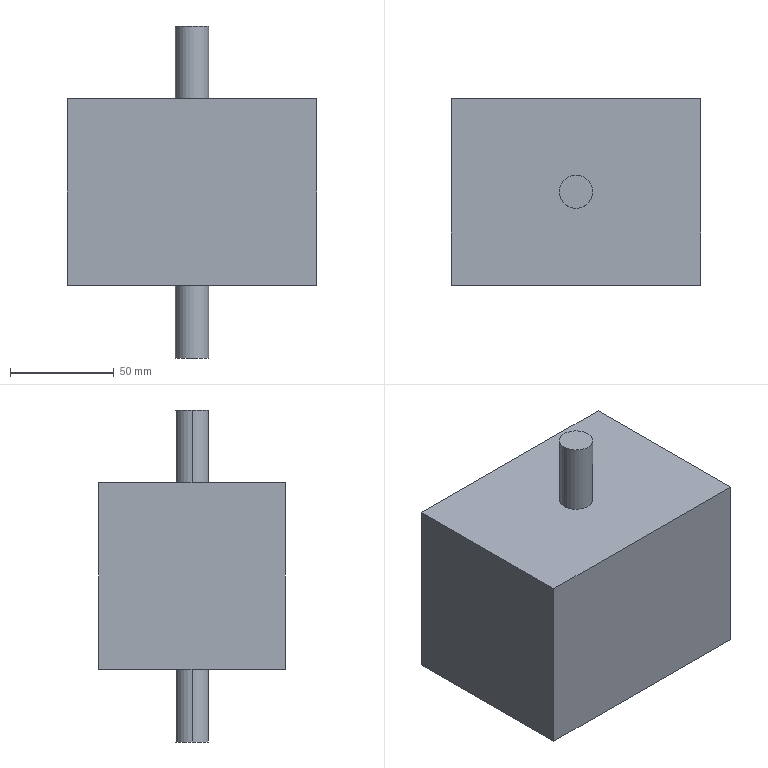Part | SolidWorks | features Extrusion 1, ICE 1 | 1 solid | 12 faces | box 120 x 90 x 160 mm | volume 986074 mm3 | plane 8 | cylinder 4 | commonest cylinder face diameters 16 x4
STEP:
#1=CARTESIAN_POINT('',(8.,0.,-80.));
#2=VERTEX_POINT('',#1);
#3=CARTESIAN_POINT('',(-8.,0.,-80.));
#4=VERTEX_POINT('',#3);
#5=CARTESIAN_POINT('',(0.,0.,-80.));
#6=DIRECTION('',(0.,0.,1.));
#7=DIRECTION('',(1.,0.,0.));
#8=AXIS2_PLACEMENT_3D('',#5,#6,#7);
#9=CIRCLE('',#8,8.);
#10=EDGE_CURVE('',#2,#4,#9,.T.);
#11=ORIENTED_EDGE('',*,*,#10,.T.);
#12=CARTESIAN_POINT('',(-8.,0.,-45.));
#13=VERTEX_POINT('',#12);
#14=CARTESIAN_POINT('',(-8.,0.,-80.));
#15=DIRECTION('',(0.,0.,1.));
#16=VECTOR('',#15,1000.);
#17=LINE('',#14,#16);
#18=EDGE_CURVE('',#4,#13,#17,.T.);
#19=ORIENTED_EDGE('',*,*,#18,.T.);
#20=CARTESIAN_POINT('',(8.,0.,-45.));
#21=VERTEX_POINT('',#20);
#22=CARTESIAN_POINT('',(0.,0.,-45.));
#23=DIRECTION('',(0.,0.,1.));
#24=DIRECTION('',(1.,0.,0.));
#25=AXIS2_PLACEMENT_3D('',#22,#23,#24);
#26=CIRCLE('',#25,8.);
#27=EDGE_CURVE('',#21,#13,#26,.T.);
#28=ORIENTED_EDGE('',*,*,#27,.F.);
#29=CARTESIAN_POINT('',(8.,0.,-80.));
#30=DIRECTION('',(0.,0.,1.));
#31=VECTOR('',#30,1000.);
#32=LINE('',#29,#31);
#33=EDGE_CURVE('',#2,#21,#32,.T.);
#34=ORIENTED_EDGE('',*,*,#33,.F.);
#35=EDGE_LOOP('',(#11,#19,#28,#34));
#36=FACE_OUTER_BOUND('',#35,.T.);
#37=CARTESIAN_POINT('',(0.,0.,-80.));
#38=DIRECTION('',(0.,0.,1.));
#39=DIRECTION('',(1.,0.,0.));
#40=AXIS2_PLACEMENT_3D('',#37,#38,#39);
#41=CYLINDRICAL_SURFACE('',#40,8.);
#42=ADVANCED_FACE('',(#36),#41,.T.);
#43=CARTESIAN_POINT('',(8.,0.,45.));
#44=VERTEX_POINT('',#43);
#45=CARTESIAN_POINT('',(-8.,0.,45.));
#46=VERTEX_POINT('',#45);
#47=CARTESIAN_POINT('',(0.,0.,45.));
#48=DIRECTION('',(0.,0.,1.));
#49=DIRECTION('',(1.,0.,0.));
#50=AXIS2_PLACEMENT_3D('',#47,#48,#49);
#51=CIRCLE('',#50,8.);
#52=EDGE_CURVE('',#44,#46,#51,.T.);
#53=ORIENTED_EDGE('',*,*,#52,.T.);
#54=CARTESIAN_POINT('',(-8.,0.,80.));
#55=VERTEX_POINT('',#54);
#56=CARTESIAN_POINT('',(-8.,0.,-80.));
#57=DIRECTION('',(0.,0.,1.));
#58=VECTOR('',#57,1000.);
#59=LINE('',#56,#58);
#60=EDGE_CURVE('',#46,#55,#59,.T.);
#61=ORIENTED_EDGE('',*,*,#60,.T.);
#62=CARTESIAN_POINT('',(8.,0.,80.));
#63=VERTEX_POINT('',#62);
#64=CARTESIAN_POINT('',(0.,0.,80.));
#65=DIRECTION('',(0.,0.,1.));
#66=DIRECTION('',(1.,0.,0.));
#67=AXIS2_PLACEMENT_3D('',#64,#65,#66);
#68=CIRCLE('',#67,8.);
#69=EDGE_CURVE('',#63,#55,#68,.T.);
#70=ORIENTED_EDGE('',*,*,#69,.F.);
#71=CARTESIAN_POINT('',(8.,0.,-80.));
#72=DIRECTION('',(0.,0.,1.));
#73=VECTOR('',#72,1000.);
#74=LINE('',#71,#73);
#75=EDGE_CURVE('',#44,#63,#74,.T.);
#76=ORIENTED_EDGE('',*,*,#75,.F.);
#77=EDGE_LOOP('',(#53,#61,#70,#76));
#78=FACE_OUTER_BOUND('',#77,.T.);
#79=CARTESIAN_POINT('',(0.,0.,-80.));
#80=DIRECTION('',(0.,0.,1.));
#81=DIRECTION('',(1.,0.,0.));
#82=AXIS2_PLACEMENT_3D('',#79,#80,#81);
#83=CYLINDRICAL_SURFACE('',#82,8.);
#84=ADVANCED_FACE('',(#78),#83,.T.);
#85=CARTESIAN_POINT('',(-60.,45.,45.));
#86=VERTEX_POINT('',#85);
#87=CARTESIAN_POINT('',(-60.,-45.,45.));
#88=VERTEX_POINT('',#87);
#89=CARTESIAN_POINT('',(-60.,45.,45.));
#90=DIRECTION('',(0.,-1.,0.));
#91=VECTOR('',#90,1000.);
#92=LINE('',#89,#91);
#93=EDGE_CURVE('',#86,#88,#92,.T.);
#94=ORIENTED_EDGE('',*,*,#93,.F.);
#95=CARTESIAN_POINT('',(-60.,45.,-45.));
#96=VERTEX_POINT('',#95);
#97=CARTESIAN_POINT('',(-60.,45.,-45.));
#98=DIRECTION('',(0.,0.,1.));
#99=VECTOR('',#98,1000.);
#100=LINE('',#97,#99);
#101=EDGE_CURVE('',#96,#86,#100,.T.);
#102=ORIENTED_EDGE('',*,*,#101,.F.);
#103=CARTESIAN_POINT('',(-60.,-45.,-45.));
#104=VERTEX_POINT('',#103);
#105=CARTESIAN_POINT('',(-60.,45.,-45.));
#106=DIRECTION('',(0.,-1.,0.));
#107=VECTOR('',#106,1000.);
#108=LINE('',#105,#107);
#109=EDGE_CURVE('',#96,#104,#108,.T.);
#110=ORIENTED_EDGE('',*,*,#109,.T.);
#111=CARTESIAN_POINT('',(-60.,-45.,-45.));
#112=DIRECTION('',(0.,0.,1.));
#113=VECTOR('',#112,1000.);
#114=LINE('',#111,#113);
#115=EDGE_CURVE('',#104,#88,#114,.T.);
#116=ORIENTED_EDGE('',*,*,#115,.T.);
#117=EDGE_LOOP('',(#94,#102,#110,#116));
#118=FACE_OUTER_BOUND('',#117,.T.);
#119=CARTESIAN_POINT('',(-60.,45.,-45.));
#120=DIRECTION('',(-1.,0.,0.));
#121=DIRECTION('',(0.,0.,1.));
#122=AXIS2_PLACEMENT_3D('',#119,#120,#121);
#123=PLANE('',#122);
#124=ADVANCED_FACE('',(#118),#123,.T.);
#125=CARTESIAN_POINT('',(60.,45.,45.));
#126=VERTEX_POINT('',#125);
#127=CARTESIAN_POINT('',(60.,45.,45.));
#128=DIRECTION('',(-1.,0.,0.));
#129=VECTOR('',#128,1000.);
#130=LINE('',#127,#129);
#131=EDGE_CURVE('',#126,#86,#130,.T.);
#132=ORIENTED_EDGE('',*,*,#131,.F.);
#133=CARTESIAN_POINT('',(60.,45.,-45.));
#134=VERTEX_POINT('',#133);
#135=CARTESIAN_POINT('',(60.,45.,-45.));
#136=DIRECTION('',(0.,0.,1.));
#137=VECTOR('',#136,1000.);
#138=LINE('',#135,#137);
#139=EDGE_CURVE('',#134,#126,#138,.T.);
#140=ORIENTED_EDGE('',*,*,#139,.F.);
#141=CARTESIAN_POINT('',(60.,45.,-45.));
#142=DIRECTION('',(-1.,0.,0.));
#143=VECTOR('',#142,1000.);
#144=LINE('',#141,#143);
#145=EDGE_CURVE('',#134,#96,#144,.T.);
#146=ORIENTED_EDGE('',*,*,#145,.T.);
#147=ORIENTED_EDGE('',*,*,#101,.T.);
#148=EDGE_LOOP('',(#132,#140,#146,#147));
#149=FACE_OUTER_BOUND('',#148,.T.);
#150=CARTESIAN_POINT('',(60.,45.,-45.));
#151=DIRECTION('',(0.,1.,0.));
#152=DIRECTION('',(0.,0.,1.));
#153=AXIS2_PLACEMENT_3D('',#150,#151,#152);
#154=PLANE('',#153);
#155=ADVANCED_FACE('',(#149),#154,.T.);
#156=CARTESIAN_POINT('',(60.,-45.,45.));
#157=VERTEX_POINT('',#156);
#158=CARTESIAN_POINT('',(60.,-45.,45.));
#159=DIRECTION('',(0.,1.,0.));
#160=VECTOR('',#159,1000.);
#161=LINE('',#158,#160);
#162=EDGE_CURVE('',#157,#126,#161,.T.);
#163=ORIENTED_EDGE('',*,*,#162,.F.);
#164=CARTESIAN_POINT('',(60.,-45.,-45.));
#165=VERTEX_POINT('',#164);
#166=CARTESIAN_POINT('',(60.,-45.,-45.));
#167=DIRECTION('',(0.,0.,1.));
#168=VECTOR('',#167,1000.);
#169=LINE('',#166,#168);
#170=EDGE_CURVE('',#165,#157,#169,.T.);
#171=ORIENTED_EDGE('',*,*,#170,.F.);
#172=CARTESIAN_POINT('',(60.,-45.,-45.));
#173=DIRECTION('',(0.,1.,0.));
#174=VECTOR('',#173,1000.);
#175=LINE('',#172,#174);
#176=EDGE_CURVE('',#165,#134,#175,.T.);
#177=ORIENTED_EDGE('',*,*,#176,.T.);
#178=ORIENTED_EDGE('',*,*,#139,.T.);
#179=EDGE_LOOP('',(#163,#171,#177,#178));
#180=FACE_OUTER_BOUND('',#179,.T.);
#181=CARTESIAN_POINT('',(60.,-45.,-45.));
#182=DIRECTION('',(1.,0.,0.));
#183=DIRECTION('',(0.,0.,-1.));
#184=AXIS2_PLACEMENT_3D('',#181,#182,#183);
#185=PLANE('',#184);
#186=ADVANCED_FACE('',(#180),#185,.T.);
#187=CARTESIAN_POINT('',(-60.,-45.,45.));
#188=DIRECTION('',(1.,0.,0.));
#189=VECTOR('',#188,1000.);
#190=LINE('',#187,#189);
#191=EDGE_CURVE('',#88,#157,#190,.T.);
#192=ORIENTED_EDGE('',*,*,#191,.F.);
#193=ORIENTED_EDGE('',*,*,#115,.F.);
#194=CARTESIAN_POINT('',(-60.,-45.,-45.));
#195=DIRECTION('',(1.,0.,0.));
#196=VECTOR('',#195,1000.);
#197=LINE('',#194,#196);
#198=EDGE_CURVE('',#104,#165,#197,.T.);
#199=ORIENTED_EDGE('',*,*,#198,.T.);
#200=ORIENTED_EDGE('',*,*,#170,.T.);
#201=EDGE_LOOP('',(#192,#193,#199,#200));
#202=FACE_OUTER_BOUND('',#201,.T.);
#203=CARTESIAN_POINT('',(-60.,-45.,-45.));
#204=DIRECTION('',(0.,-1.,0.));
#205=DIRECTION('',(0.,0.,-1.));
#206=AXIS2_PLACEMENT_3D('',#203,#204,#205);
#207=PLANE('',#206);
#208=ADVANCED_FACE('',(#202),#207,.T.);
#209=ORIENTED_EDGE('',*,*,#27,.T.);
#210=CARTESIAN_POINT('',(0.,0.,-45.));
#211=DIRECTION('',(0.,0.,1.));
#212=DIRECTION('',(1.,0.,0.));
#213=AXIS2_PLACEMENT_3D('',#210,#211,#212);
#214=CIRCLE('',#213,8.);
#215=EDGE_CURVE('',#13,#21,#214,.T.);
#216=ORIENTED_EDGE('',*,*,#215,.T.);
#217=EDGE_LOOP('',(#209,#216));
#218=FACE_BOUND('',#217,.T.);
#219=ORIENTED_EDGE('',*,*,#109,.F.);
#220=ORIENTED_EDGE('',*,*,#145,.F.);
#221=ORIENTED_EDGE('',*,*,#176,.F.);
#222=ORIENTED_EDGE('',*,*,#198,.F.);
#223=EDGE_LOOP('',(#219,#220,#221,#222));
#224=FACE_OUTER_BOUND('',#223,.T.);
#225=CARTESIAN_POINT('',(0.,0.,-45.));
#226=DIRECTION('',(0.,0.,1.));
#227=DIRECTION('',(1.,0.,0.));
#228=AXIS2_PLACEMENT_3D('',#225,#226,#227);
#229=PLANE('',#228);
#230=ADVANCED_FACE('',(#218,#224),#229,.F.);
#231=ORIENTED_EDGE('',*,*,#52,.F.);
#232=CARTESIAN_POINT('',(0.,0.,45.));
#233=DIRECTION('',(0.,0.,1.));
#234=DIRECTION('',(1.,0.,0.));
#235=AXIS2_PLACEMENT_3D('',#232,#233,#234);
#236=CIRCLE('',#235,8.);
#237=EDGE_CURVE('',#46,#44,#236,.T.);
#238=ORIENTED_EDGE('',*,*,#237,.F.);
#239=EDGE_LOOP('',(#231,#238));
#240=FACE_BOUND('',#239,.T.);
#241=ORIENTED_EDGE('',*,*,#93,.T.);
#242=ORIENTED_EDGE('',*,*,#191,.T.);
#243=ORIENTED_EDGE('',*,*,#162,.T.);
#244=ORIENTED_EDGE('',*,*,#131,.T.);
#245=EDGE_LOOP('',(#241,#242,#243,#244));
#246=FACE_OUTER_BOUND('',#245,.T.);
#247=CARTESIAN_POINT('',(0.,0.,45.));
#248=DIRECTION('',(0.,0.,1.));
#249=DIRECTION('',(1.,0.,0.));
#250=AXIS2_PLACEMENT_3D('',#247,#248,#249);
#251=PLANE('',#250);
#252=ADVANCED_FACE('',(#240,#246),#251,.T.);
#253=ORIENTED_EDGE('',*,*,#69,.T.);
#254=CARTESIAN_POINT('',(0.,0.,80.));
#255=DIRECTION('',(0.,0.,1.));
#256=DIRECTION('',(1.,0.,0.));
#257=AXIS2_PLACEMENT_3D('',#254,#255,#256);
#258=CIRCLE('',#257,8.);
#259=EDGE_CURVE('',#55,#63,#258,.T.);
#260=ORIENTED_EDGE('',*,*,#259,.T.);
#261=EDGE_LOOP('',(#253,#260));
#262=FACE_OUTER_BOUND('',#261,.T.);
#263=CARTESIAN_POINT('',(0.,0.,80.));
#264=DIRECTION('',(0.,0.,1.));
#265=DIRECTION('',(1.,0.,0.));
#266=AXIS2_PLACEMENT_3D('',#263,#264,#265);
#267=PLANE('',#266);
#268=ADVANCED_FACE('',(#262),#267,.T.);
#269=ORIENTED_EDGE('',*,*,#60,.F.);
#270=ORIENTED_EDGE('',*,*,#237,.T.);
#271=ORIENTED_EDGE('',*,*,#75,.T.);
#272=ORIENTED_EDGE('',*,*,#259,.F.);
#273=EDGE_LOOP('',(#269,#270,#271,#272));
#274=FACE_OUTER_BOUND('',#273,.T.);
#275=CARTESIAN_POINT('',(0.,0.,-80.));
#276=DIRECTION('',(0.,0.,1.));
#277=DIRECTION('',(1.,0.,0.));
#278=AXIS2_PLACEMENT_3D('',#275,#276,#277);
#279=CYLINDRICAL_SURFACE('',#278,8.);
#280=ADVANCED_FACE('',(#274),#279,.T.);
#281=ORIENTED_EDGE('',*,*,#18,.F.);
#282=CARTESIAN_POINT('',(0.,0.,-80.));
#283=DIRECTION('',(0.,0.,1.));
#284=DIRECTION('',(1.,0.,0.));
#285=AXIS2_PLACEMENT_3D('',#282,#283,#284);
#286=CIRCLE('',#285,8.);
#287=EDGE_CURVE('',#4,#2,#286,.T.);
#288=ORIENTED_EDGE('',*,*,#287,.T.);
#289=ORIENTED_EDGE('',*,*,#33,.T.);
#290=ORIENTED_EDGE('',*,*,#215,.F.);
#291=EDGE_LOOP('',(#281,#288,#289,#290));
#292=FACE_OUTER_BOUND('',#291,.T.);
#293=CARTESIAN_POINT('',(0.,0.,-80.));
#294=DIRECTION('',(0.,0.,1.));
#295=DIRECTION('',(1.,0.,0.));
#296=AXIS2_PLACEMENT_3D('',#293,#294,#295);
#297=CYLINDRICAL_SURFACE('',#296,8.);
#298=ADVANCED_FACE('',(#292),#297,.T.);
#299=ORIENTED_EDGE('',*,*,#10,.F.);
#300=ORIENTED_EDGE('',*,*,#287,.F.);
#301=EDGE_LOOP('',(#299,#300));
#302=FACE_OUTER_BOUND('',#301,.T.);
#303=CARTESIAN_POINT('',(0.,0.,-80.));
#304=DIRECTION('',(0.,0.,1.));
#305=DIRECTION('',(1.,0.,0.));
#306=AXIS2_PLACEMENT_3D('',#303,#304,#305);
#307=PLANE('',#306);
#308=ADVANCED_FACE('',(#302),#307,.F.);
#309=CLOSED_SHELL('',(#42,#84,#124,#155,#186,#208,#230,#252,#268,#280,#298,#308));
#310=MANIFOLD_SOLID_BREP('',#309);
#311=CARTESIAN_POINT('',(0.,0.,0.));
#312=DIRECTION('',(0.,0.,1.));
#313=DIRECTION('',(1.,0.,0.));
#314=AXIS2_PLACEMENT_3D('',#311,#312,#313);
#315=(LENGTH_UNIT()NAMED_UNIT(*)SI_UNIT(.MILLI.,.METRE.));
#316=UNCERTAINTY_MEASURE_WITH_UNIT(LENGTH_MEASURE(0.00001),#315,'','');
#317=(NAMED_UNIT(*)PLANE_ANGLE_UNIT()SI_UNIT($,.RADIAN.));
#318=(NAMED_UNIT(*)SI_UNIT($,.STERADIAN.)SOLID_ANGLE_UNIT());
#319=(GEOMETRIC_REPRESENTATION_CONTEXT(3)GLOBAL_UNCERTAINTY_ASSIGNED_CONTEXT((#316))GLOBAL_UNIT_ASSIGNED_CONTEXT((#315,#317,#318))REPRESENTATION_CONTEXT('',''));
#320=ADVANCED_BREP_SHAPE_REPRESENTATION('',(#310,#314),#319);